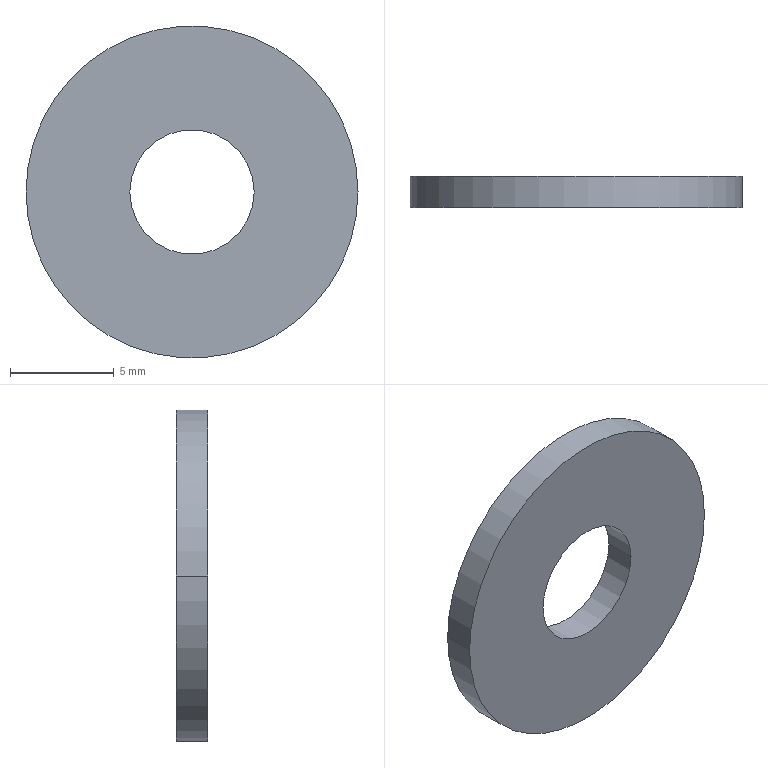Part | STEP file | WSSS16-6-1.5-3 | 1 solid | 6 faces | box 16 x 1.5 x 16 mm | volume 259.181 mm3 | cylinder 4 | plane 2 | commonest cylinder face diameters 6 x2 16 x2
STEP:
#1=CARTESIAN_POINT('',(0.,0.,0.));
#2=DIRECTION('',(0.,0.,1.));
#3=DIRECTION('',(1.,0.,0.));
#4=AXIS2_PLACEMENT_3D('',#1,#2,#3);
#5=CARTESIAN_POINT('',(-3.,0.,0.));
#6=VERTEX_POINT('',#5);
#7=CARTESIAN_POINT('',(-3.,1.5,0.));
#8=VERTEX_POINT('',#7);
#9=CARTESIAN_POINT('',(-3.,0.,0.));
#10=DIRECTION('',(0.,1.,0.));
#11=VECTOR('',#10,1.);
#12=LINE('',#9,#11);
#13=CARTESIAN_POINT('',(0.,0.,0.));
#14=DIRECTION('',(0.,1.,0.));
#15=DIRECTION('',(-1.,0.,0.));
#16=AXIS2_PLACEMENT_3D('',#13,#14,#15);
#17=CYLINDRICAL_SURFACE('',#16,3.);
#18=CARTESIAN_POINT('',(6.283,0.));
#19=DIRECTION('',(0.,1.));
#20=VECTOR('',#19,1.);
#21=LINE('',#18,#20);
#22=(GEOMETRIC_REPRESENTATION_CONTEXT(2)PARAMETRIC_REPRESENTATION_CONTEXT()REPRESENTATION_CONTEXT('',''));
#23=DEFINITIONAL_REPRESENTATION('',(#21),#22);
#24=PCURVE('',#17,#23);
#25=CARTESIAN_POINT('',(0.,0.,0.));
#26=DIRECTION('',(0.,1.,0.));
#27=DIRECTION('',(-1.,0.,0.));
#28=AXIS2_PLACEMENT_3D('',#25,#26,#27);
#29=CYLINDRICAL_SURFACE('',#28,3.);
#30=CARTESIAN_POINT('',(0.,0.));
#31=DIRECTION('',(0.,1.));
#32=VECTOR('',#31,1.);
#33=LINE('',#30,#32);
#34=(GEOMETRIC_REPRESENTATION_CONTEXT(2)PARAMETRIC_REPRESENTATION_CONTEXT()REPRESENTATION_CONTEXT('',''));
#35=DEFINITIONAL_REPRESENTATION('',(#33),#34);
#36=PCURVE('',#29,#35);
#37=SURFACE_CURVE('',#12,(#24,#36),.PCURVE_S1.);
#38=EDGE_CURVE('',#6,#8,#37,.T.);
#39=ORIENTED_EDGE('',*,*,#38,.T.);
#40=CARTESIAN_POINT('',(3.,1.5,0.));
#41=VERTEX_POINT('',#40);
#42=CARTESIAN_POINT('',(0.,1.5,0.));
#43=DIRECTION('',(0.,-1.,0.));
#44=DIRECTION('',(1.,0.,0.));
#45=AXIS2_PLACEMENT_3D('',#42,#43,#44);
#46=CIRCLE('',#45,3.);
#47=CARTESIAN_POINT('',(9.425,1.5));
#48=DIRECTION('',(-1.,0.));
#49=VECTOR('',#48,1.);
#50=LINE('',#47,#49);
#51=(GEOMETRIC_REPRESENTATION_CONTEXT(2)PARAMETRIC_REPRESENTATION_CONTEXT()REPRESENTATION_CONTEXT('',''));
#52=DEFINITIONAL_REPRESENTATION('',(#50),#51);
#53=PCURVE('',#17,#52);
#54=CARTESIAN_POINT('',(0.,1.5,0.));
#55=DIRECTION('',(0.,1.,0.));
#56=DIRECTION('',(-1.,0.,0.));
#57=AXIS2_PLACEMENT_3D('',#54,#55,#56);
#58=PLANE('',#57);
#59=CARTESIAN_POINT('',(-3.,0.));
#60=CARTESIAN_POINT('',(-3.,5.196));
#61=CARTESIAN_POINT('',(1.5,2.598));
#62=CARTESIAN_POINT('',(6.,0.));
#63=CARTESIAN_POINT('',(1.5,-2.598));
#64=CARTESIAN_POINT('',(-3.,-5.196));
#65=CARTESIAN_POINT('',(-3.,0.));
#66=(BOUNDED_CURVE()B_SPLINE_CURVE(2,(#59,#60,#61,#62,#63,#64,#65),.UNSPECIFIED.,.T.,.F.)B_SPLINE_CURVE_WITH_KNOTS((1,2,2,2,2,1),(-2.094,0.,2.094,4.189,6.283,8.378),.UNSPECIFIED.)CURVE()GEOMETRIC_REPRESENTATION_ITEM()RATIONAL_B_SPLINE_CURVE((1.,0.5,1.,0.5,1.,0.5,1.))REPRESENTATION_ITEM(''));
#67=(GEOMETRIC_REPRESENTATION_CONTEXT(2)PARAMETRIC_REPRESENTATION_CONTEXT()REPRESENTATION_CONTEXT('',''));
#68=DEFINITIONAL_REPRESENTATION('',(#66),#67);
#69=PCURVE('',#58,#68);
#70=SURFACE_CURVE('',#46,(#53,#69),.PCURVE_S1.);
#71=EDGE_CURVE('',#8,#41,#70,.T.);
#72=ORIENTED_EDGE('',*,*,#71,.T.);
#73=CARTESIAN_POINT('',(3.,0.,0.));
#74=VERTEX_POINT('',#73);
#75=CARTESIAN_POINT('',(3.,0.,0.));
#76=DIRECTION('',(0.,1.,0.));
#77=VECTOR('',#76,1.);
#78=LINE('',#75,#77);
#79=CARTESIAN_POINT('',(3.142,0.));
#80=DIRECTION('',(0.,1.));
#81=VECTOR('',#80,1.);
#82=LINE('',#79,#81);
#83=(GEOMETRIC_REPRESENTATION_CONTEXT(2)PARAMETRIC_REPRESENTATION_CONTEXT()REPRESENTATION_CONTEXT('',''));
#84=DEFINITIONAL_REPRESENTATION('',(#82),#83);
#85=PCURVE('',#17,#84);
#86=CARTESIAN_POINT('',(3.142,0.));
#87=DIRECTION('',(0.,1.));
#88=VECTOR('',#87,1.);
#89=LINE('',#86,#88);
#90=(GEOMETRIC_REPRESENTATION_CONTEXT(2)PARAMETRIC_REPRESENTATION_CONTEXT()REPRESENTATION_CONTEXT('',''));
#91=DEFINITIONAL_REPRESENTATION('',(#89),#90);
#92=PCURVE('',#29,#91);
#93=SURFACE_CURVE('',#78,(#85,#92),.PCURVE_S1.);
#94=EDGE_CURVE('',#74,#41,#93,.T.);
#95=ORIENTED_EDGE('',*,*,#94,.F.);
#96=CARTESIAN_POINT('',(0.,0.,0.));
#97=DIRECTION('',(0.,1.,0.));
#98=DIRECTION('',(-1.,0.,0.));
#99=AXIS2_PLACEMENT_3D('',#96,#97,#98);
#100=CIRCLE('',#99,3.);
#101=CARTESIAN_POINT('',(0.,0.));
#102=DIRECTION('',(1.,0.));
#103=VECTOR('',#102,1.);
#104=LINE('',#101,#103);
#105=(GEOMETRIC_REPRESENTATION_CONTEXT(2)PARAMETRIC_REPRESENTATION_CONTEXT()REPRESENTATION_CONTEXT('',''));
#106=DEFINITIONAL_REPRESENTATION('',(#104),#105);
#107=PCURVE('',#17,#106);
#108=CARTESIAN_POINT('',(0.,0.,0.));
#109=DIRECTION('',(0.,-1.,0.));
#110=DIRECTION('',(1.,0.,0.));
#111=AXIS2_PLACEMENT_3D('',#108,#109,#110);
#112=PLANE('',#111);
#113=CARTESIAN_POINT('',(-3.,0.));
#114=CARTESIAN_POINT('',(-3.,5.196));
#115=CARTESIAN_POINT('',(1.5,2.598));
#116=CARTESIAN_POINT('',(6.,0.));
#117=CARTESIAN_POINT('',(1.5,-2.598));
#118=CARTESIAN_POINT('',(-3.,-5.196));
#119=CARTESIAN_POINT('',(-3.,0.));
#120=(BOUNDED_CURVE()B_SPLINE_CURVE(2,(#113,#114,#115,#116,#117,#118,#119),.UNSPECIFIED.,.T.,.F.)B_SPLINE_CURVE_WITH_KNOTS((1,2,2,2,2,1),(-2.094,0.,2.094,4.189,6.283,8.378),.UNSPECIFIED.)CURVE()GEOMETRIC_REPRESENTATION_ITEM()RATIONAL_B_SPLINE_CURVE((1.,0.5,1.,0.5,1.,0.5,1.))REPRESENTATION_ITEM(''));
#121=(GEOMETRIC_REPRESENTATION_CONTEXT(2)PARAMETRIC_REPRESENTATION_CONTEXT()REPRESENTATION_CONTEXT('',''));
#122=DEFINITIONAL_REPRESENTATION('',(#120),#121);
#123=PCURVE('',#112,#122);
#124=SURFACE_CURVE('',#100,(#107,#123),.PCURVE_S1.);
#125=EDGE_CURVE('',#74,#6,#124,.T.);
#126=ORIENTED_EDGE('',*,*,#125,.T.);
#127=EDGE_LOOP('',(#39,#72,#95,#126));
#128=FACE_BOUND('',#127,.F.);
#129=ADVANCED_FACE('',(#128),#17,.F.);
#130=CARTESIAN_POINT('',(-8.,0.,0.));
#131=VERTEX_POINT('',#130);
#132=CARTESIAN_POINT('',(8.,0.,0.));
#133=VERTEX_POINT('',#132);
#134=CARTESIAN_POINT('',(0.,0.,0.));
#135=DIRECTION('',(0.,1.,0.));
#136=DIRECTION('',(-1.,0.,0.));
#137=AXIS2_PLACEMENT_3D('',#134,#135,#136);
#138=CIRCLE('',#137,8.);
#139=CARTESIAN_POINT('',(0.,0.,0.));
#140=DIRECTION('',(0.,1.,0.));
#141=DIRECTION('',(-1.,0.,0.));
#142=AXIS2_PLACEMENT_3D('',#139,#140,#141);
#143=CYLINDRICAL_SURFACE('',#142,8.);
#144=CARTESIAN_POINT('',(0.,0.));
#145=DIRECTION('',(1.,0.));
#146=VECTOR('',#145,1.);
#147=LINE('',#144,#146);
#148=(GEOMETRIC_REPRESENTATION_CONTEXT(2)PARAMETRIC_REPRESENTATION_CONTEXT()REPRESENTATION_CONTEXT('',''));
#149=DEFINITIONAL_REPRESENTATION('',(#147),#148);
#150=PCURVE('',#143,#149);
#151=CARTESIAN_POINT('',(-8.,0.));
#152=CARTESIAN_POINT('',(-8.,13.856));
#153=CARTESIAN_POINT('',(4.,6.928));
#154=CARTESIAN_POINT('',(16.,0.));
#155=CARTESIAN_POINT('',(4.,-6.928));
#156=CARTESIAN_POINT('',(-8.,-13.856));
#157=CARTESIAN_POINT('',(-8.,0.));
#158=(BOUNDED_CURVE()B_SPLINE_CURVE(2,(#151,#152,#153,#154,#155,#156,#157),.UNSPECIFIED.,.T.,.F.)B_SPLINE_CURVE_WITH_KNOTS((1,2,2,2,2,1),(-2.094,0.,2.094,4.189,6.283,8.378),.UNSPECIFIED.)CURVE()GEOMETRIC_REPRESENTATION_ITEM()RATIONAL_B_SPLINE_CURVE((1.,0.5,1.,0.5,1.,0.5,1.))REPRESENTATION_ITEM(''));
#159=(GEOMETRIC_REPRESENTATION_CONTEXT(2)PARAMETRIC_REPRESENTATION_CONTEXT()REPRESENTATION_CONTEXT('',''));
#160=DEFINITIONAL_REPRESENTATION('',(#158),#159);
#161=PCURVE('',#112,#160);
#162=SURFACE_CURVE('',#138,(#150,#161),.PCURVE_S1.);
#163=EDGE_CURVE('',#131,#133,#162,.T.);
#164=ORIENTED_EDGE('',*,*,#163,.T.);
#165=CARTESIAN_POINT('',(8.,1.5,0.));
#166=VERTEX_POINT('',#165);
#167=CARTESIAN_POINT('',(8.,0.,0.));
#168=DIRECTION('',(0.,1.,0.));
#169=VECTOR('',#168,1.);
#170=LINE('',#167,#169);
#171=CARTESIAN_POINT('',(3.142,0.));
#172=DIRECTION('',(0.,1.));
#173=VECTOR('',#172,1.);
#174=LINE('',#171,#173);
#175=(GEOMETRIC_REPRESENTATION_CONTEXT(2)PARAMETRIC_REPRESENTATION_CONTEXT()REPRESENTATION_CONTEXT('',''));
#176=DEFINITIONAL_REPRESENTATION('',(#174),#175);
#177=PCURVE('',#143,#176);
#178=CARTESIAN_POINT('',(0.,0.,0.));
#179=DIRECTION('',(0.,1.,0.));
#180=DIRECTION('',(-1.,0.,0.));
#181=AXIS2_PLACEMENT_3D('',#178,#179,#180);
#182=CYLINDRICAL_SURFACE('',#181,8.);
#183=CARTESIAN_POINT('',(3.142,0.));
#184=DIRECTION('',(0.,1.));
#185=VECTOR('',#184,1.);
#186=LINE('',#183,#185);
#187=(GEOMETRIC_REPRESENTATION_CONTEXT(2)PARAMETRIC_REPRESENTATION_CONTEXT()REPRESENTATION_CONTEXT('',''));
#188=DEFINITIONAL_REPRESENTATION('',(#186),#187);
#189=PCURVE('',#182,#188);
#190=SURFACE_CURVE('',#170,(#177,#189),.PCURVE_S1.);
#191=EDGE_CURVE('',#133,#166,#190,.T.);
#192=ORIENTED_EDGE('',*,*,#191,.T.);
#193=CARTESIAN_POINT('',(-8.,1.5,0.));
#194=VERTEX_POINT('',#193);
#195=CARTESIAN_POINT('',(0.,1.5,0.));
#196=DIRECTION('',(0.,-1.,0.));
#197=DIRECTION('',(1.,0.,0.));
#198=AXIS2_PLACEMENT_3D('',#195,#196,#197);
#199=CIRCLE('',#198,8.);
#200=CARTESIAN_POINT('',(3.142,1.5));
#201=DIRECTION('',(-1.,0.));
#202=VECTOR('',#201,1.);
#203=LINE('',#200,#202);
#204=(GEOMETRIC_REPRESENTATION_CONTEXT(2)PARAMETRIC_REPRESENTATION_CONTEXT()REPRESENTATION_CONTEXT('',''));
#205=DEFINITIONAL_REPRESENTATION('',(#203),#204);
#206=PCURVE('',#143,#205);
#207=CARTESIAN_POINT('',(-8.,0.));
#208=CARTESIAN_POINT('',(-8.,13.856));
#209=CARTESIAN_POINT('',(4.,6.928));
#210=CARTESIAN_POINT('',(16.,0.));
#211=CARTESIAN_POINT('',(4.,-6.928));
#212=CARTESIAN_POINT('',(-8.,-13.856));
#213=CARTESIAN_POINT('',(-8.,0.));
#214=(BOUNDED_CURVE()B_SPLINE_CURVE(2,(#207,#208,#209,#210,#211,#212,#213),.UNSPECIFIED.,.T.,.F.)B_SPLINE_CURVE_WITH_KNOTS((1,2,2,2,2,1),(-2.094,0.,2.094,4.189,6.283,8.378),.UNSPECIFIED.)CURVE()GEOMETRIC_REPRESENTATION_ITEM()RATIONAL_B_SPLINE_CURVE((1.,0.5,1.,0.5,1.,0.5,1.))REPRESENTATION_ITEM(''));
#215=(GEOMETRIC_REPRESENTATION_CONTEXT(2)PARAMETRIC_REPRESENTATION_CONTEXT()REPRESENTATION_CONTEXT('',''));
#216=DEFINITIONAL_REPRESENTATION('',(#214),#215);
#217=PCURVE('',#58,#216);
#218=SURFACE_CURVE('',#199,(#206,#217),.PCURVE_S1.);
#219=EDGE_CURVE('',#166,#194,#218,.T.);
#220=ORIENTED_EDGE('',*,*,#219,.T.);
#221=CARTESIAN_POINT('',(-8.,0.,0.));
#222=DIRECTION('',(0.,1.,0.));
#223=VECTOR('',#222,1.);
#224=LINE('',#221,#223);
#225=CARTESIAN_POINT('',(0.,0.));
#226=DIRECTION('',(0.,1.));
#227=VECTOR('',#226,1.);
#228=LINE('',#225,#227);
#229=(GEOMETRIC_REPRESENTATION_CONTEXT(2)PARAMETRIC_REPRESENTATION_CONTEXT()REPRESENTATION_CONTEXT('',''));
#230=DEFINITIONAL_REPRESENTATION('',(#228),#229);
#231=PCURVE('',#143,#230);
#232=CARTESIAN_POINT('',(6.283,0.));
#233=DIRECTION('',(0.,1.));
#234=VECTOR('',#233,1.);
#235=LINE('',#232,#234);
#236=(GEOMETRIC_REPRESENTATION_CONTEXT(2)PARAMETRIC_REPRESENTATION_CONTEXT()REPRESENTATION_CONTEXT('',''));
#237=DEFINITIONAL_REPRESENTATION('',(#235),#236);
#238=PCURVE('',#182,#237);
#239=SURFACE_CURVE('',#224,(#231,#238),.PCURVE_S1.);
#240=EDGE_CURVE('',#131,#194,#239,.T.);
#241=ORIENTED_EDGE('',*,*,#240,.F.);
#242=EDGE_LOOP('',(#164,#192,#220,#241));
#243=FACE_BOUND('',#242,.T.);
#244=ADVANCED_FACE('',(#243),#143,.T.);
#245=ORIENTED_EDGE('',*,*,#71,.T.);
#246=CARTESIAN_POINT('',(0.,1.5,0.));
#247=DIRECTION('',(0.,-1.,0.));
#248=DIRECTION('',(1.,0.,0.));
#249=AXIS2_PLACEMENT_3D('',#246,#247,#248);
#250=CIRCLE('',#249,3.);
#251=CARTESIAN_POINT('',(-3.,0.));
#252=CARTESIAN_POINT('',(-3.,5.196));
#253=CARTESIAN_POINT('',(1.5,2.598));
#254=CARTESIAN_POINT('',(6.,0.));
#255=CARTESIAN_POINT('',(1.5,-2.598));
#256=CARTESIAN_POINT('',(-3.,-5.196));
#257=CARTESIAN_POINT('',(-3.,0.));
#258=(BOUNDED_CURVE()B_SPLINE_CURVE(2,(#251,#252,#253,#254,#255,#256,#257),.UNSPECIFIED.,.T.,.F.)B_SPLINE_CURVE_WITH_KNOTS((1,2,2,2,2,1),(-2.094,0.,2.094,4.189,6.283,8.378),.UNSPECIFIED.)CURVE()GEOMETRIC_REPRESENTATION_ITEM()RATIONAL_B_SPLINE_CURVE((1.,0.5,1.,0.5,1.,0.5,1.))REPRESENTATION_ITEM(''));
#259=(GEOMETRIC_REPRESENTATION_CONTEXT(2)PARAMETRIC_REPRESENTATION_CONTEXT()REPRESENTATION_CONTEXT('',''));
#260=DEFINITIONAL_REPRESENTATION('',(#258),#259);
#261=PCURVE('',#58,#260);
#262=CARTESIAN_POINT('',(3.142,1.5));
#263=DIRECTION('',(-1.,0.));
#264=VECTOR('',#263,1.);
#265=LINE('',#262,#264);
#266=(GEOMETRIC_REPRESENTATION_CONTEXT(2)PARAMETRIC_REPRESENTATION_CONTEXT()REPRESENTATION_CONTEXT('',''));
#267=DEFINITIONAL_REPRESENTATION('',(#265),#266);
#268=PCURVE('',#29,#267);
#269=SURFACE_CURVE('',#250,(#261,#268),.PCURVE_S1.);
#270=EDGE_CURVE('',#41,#8,#269,.T.);
#271=ORIENTED_EDGE('',*,*,#270,.T.);
#272=EDGE_LOOP('',(#245,#271));
#273=FACE_BOUND('',#272,.T.);
#274=CARTESIAN_POINT('',(0.,1.5,0.));
#275=DIRECTION('',(0.,-1.,0.));
#276=DIRECTION('',(1.,0.,0.));
#277=AXIS2_PLACEMENT_3D('',#274,#275,#276);
#278=CIRCLE('',#277,8.);
#279=CARTESIAN_POINT('',(-8.,0.));
#280=CARTESIAN_POINT('',(-8.,13.856));
#281=CARTESIAN_POINT('',(4.,6.928));
#282=CARTESIAN_POINT('',(16.,0.));
#283=CARTESIAN_POINT('',(4.,-6.928));
#284=CARTESIAN_POINT('',(-8.,-13.856));
#285=CARTESIAN_POINT('',(-8.,0.));
#286=(BOUNDED_CURVE()B_SPLINE_CURVE(2,(#279,#280,#281,#282,#283,#284,#285),.UNSPECIFIED.,.T.,.F.)B_SPLINE_CURVE_WITH_KNOTS((1,2,2,2,2,1),(-2.094,0.,2.094,4.189,6.283,8.378),.UNSPECIFIED.)CURVE()GEOMETRIC_REPRESENTATION_ITEM()RATIONAL_B_SPLINE_CURVE((1.,0.5,1.,0.5,1.,0.5,1.))REPRESENTATION_ITEM(''));
#287=(GEOMETRIC_REPRESENTATION_CONTEXT(2)PARAMETRIC_REPRESENTATION_CONTEXT()REPRESENTATION_CONTEXT('',''));
#288=DEFINITIONAL_REPRESENTATION('',(#286),#287);
#289=PCURVE('',#58,#288);
#290=CARTESIAN_POINT('',(9.425,1.5));
#291=DIRECTION('',(-1.,0.));
#292=VECTOR('',#291,1.);
#293=LINE('',#290,#292);
#294=(GEOMETRIC_REPRESENTATION_CONTEXT(2)PARAMETRIC_REPRESENTATION_CONTEXT()REPRESENTATION_CONTEXT('',''));
#295=DEFINITIONAL_REPRESENTATION('',(#293),#294);
#296=PCURVE('',#182,#295);
#297=SURFACE_CURVE('',#278,(#289,#296),.PCURVE_S1.);
#298=EDGE_CURVE('',#194,#166,#297,.T.);
#299=ORIENTED_EDGE('',*,*,#298,.F.);
#300=ORIENTED_EDGE('',*,*,#219,.F.);
#301=EDGE_LOOP('',(#299,#300));
#302=FACE_BOUND('',#301,.T.);
#303=ADVANCED_FACE('',(#273,#302),#58,.T.);
#304=CARTESIAN_POINT('',(0.,0.,0.));
#305=DIRECTION('',(0.,1.,0.));
#306=DIRECTION('',(-1.,0.,0.));
#307=AXIS2_PLACEMENT_3D('',#304,#305,#306);
#308=CIRCLE('',#307,3.);
#309=CARTESIAN_POINT('',(-3.,0.));
#310=CARTESIAN_POINT('',(-3.,5.196));
#311=CARTESIAN_POINT('',(1.5,2.598));
#312=CARTESIAN_POINT('',(6.,0.));
#313=CARTESIAN_POINT('',(1.5,-2.598));
#314=CARTESIAN_POINT('',(-3.,-5.196));
#315=CARTESIAN_POINT('',(-3.,0.));
#316=(BOUNDED_CURVE()B_SPLINE_CURVE(2,(#309,#310,#311,#312,#313,#314,#315),.UNSPECIFIED.,.T.,.F.)B_SPLINE_CURVE_WITH_KNOTS((1,2,2,2,2,1),(-2.094,0.,2.094,4.189,6.283,8.378),.UNSPECIFIED.)CURVE()GEOMETRIC_REPRESENTATION_ITEM()RATIONAL_B_SPLINE_CURVE((1.,0.5,1.,0.5,1.,0.5,1.))REPRESENTATION_ITEM(''));
#317=(GEOMETRIC_REPRESENTATION_CONTEXT(2)PARAMETRIC_REPRESENTATION_CONTEXT()REPRESENTATION_CONTEXT('',''));
#318=DEFINITIONAL_REPRESENTATION('',(#316),#317);
#319=PCURVE('',#112,#318);
#320=CARTESIAN_POINT('',(0.,0.));
#321=DIRECTION('',(1.,0.));
#322=VECTOR('',#321,1.);
#323=LINE('',#320,#322);
#324=(GEOMETRIC_REPRESENTATION_CONTEXT(2)PARAMETRIC_REPRESENTATION_CONTEXT()REPRESENTATION_CONTEXT('',''));
#325=DEFINITIONAL_REPRESENTATION('',(#323),#324);
#326=PCURVE('',#29,#325);
#327=SURFACE_CURVE('',#308,(#319,#326),.PCURVE_S1.);
#328=EDGE_CURVE('',#6,#74,#327,.T.);
#329=ORIENTED_EDGE('',*,*,#328,.T.);
#330=ORIENTED_EDGE('',*,*,#125,.T.);
#331=EDGE_LOOP('',(#329,#330));
#332=FACE_BOUND('',#331,.T.);
#333=ORIENTED_EDGE('',*,*,#163,.F.);
#334=CARTESIAN_POINT('',(0.,0.,0.));
#335=DIRECTION('',(0.,1.,0.));
#336=DIRECTION('',(-1.,0.,0.));
#337=AXIS2_PLACEMENT_3D('',#334,#335,#336);
#338=CIRCLE('',#337,8.);
#339=CARTESIAN_POINT('',(-8.,0.));
#340=CARTESIAN_POINT('',(-8.,13.856));
#341=CARTESIAN_POINT('',(4.,6.928));
#342=CARTESIAN_POINT('',(16.,0.));
#343=CARTESIAN_POINT('',(4.,-6.928));
#344=CARTESIAN_POINT('',(-8.,-13.856));
#345=CARTESIAN_POINT('',(-8.,0.));
#346=(BOUNDED_CURVE()B_SPLINE_CURVE(2,(#339,#340,#341,#342,#343,#344,#345),.UNSPECIFIED.,.T.,.F.)B_SPLINE_CURVE_WITH_KNOTS((1,2,2,2,2,1),(-2.094,0.,2.094,4.189,6.283,8.378),.UNSPECIFIED.)CURVE()GEOMETRIC_REPRESENTATION_ITEM()RATIONAL_B_SPLINE_CURVE((1.,0.5,1.,0.5,1.,0.5,1.))REPRESENTATION_ITEM(''));
#347=(GEOMETRIC_REPRESENTATION_CONTEXT(2)PARAMETRIC_REPRESENTATION_CONTEXT()REPRESENTATION_CONTEXT('',''));
#348=DEFINITIONAL_REPRESENTATION('',(#346),#347);
#349=PCURVE('',#112,#348);
#350=CARTESIAN_POINT('',(0.,0.));
#351=DIRECTION('',(1.,0.));
#352=VECTOR('',#351,1.);
#353=LINE('',#350,#352);
#354=(GEOMETRIC_REPRESENTATION_CONTEXT(2)PARAMETRIC_REPRESENTATION_CONTEXT()REPRESENTATION_CONTEXT('',''));
#355=DEFINITIONAL_REPRESENTATION('',(#353),#354);
#356=PCURVE('',#182,#355);
#357=SURFACE_CURVE('',#338,(#349,#356),.PCURVE_S1.);
#358=EDGE_CURVE('',#133,#131,#357,.T.);
#359=ORIENTED_EDGE('',*,*,#358,.F.);
#360=EDGE_LOOP('',(#333,#359));
#361=FACE_BOUND('',#360,.T.);
#362=ADVANCED_FACE('',(#332,#361),#112,.T.);
#363=ORIENTED_EDGE('',*,*,#191,.F.);
#364=ORIENTED_EDGE('',*,*,#358,.T.);
#365=ORIENTED_EDGE('',*,*,#240,.T.);
#366=ORIENTED_EDGE('',*,*,#298,.T.);
#367=EDGE_LOOP('',(#363,#364,#365,#366));
#368=FACE_BOUND('',#367,.T.);
#369=ADVANCED_FACE('',(#368),#182,.T.);
#370=ORIENTED_EDGE('',*,*,#270,.T.);
#371=ORIENTED_EDGE('',*,*,#38,.F.);
#372=ORIENTED_EDGE('',*,*,#328,.T.);
#373=ORIENTED_EDGE('',*,*,#94,.T.);
#374=EDGE_LOOP('',(#370,#371,#372,#373));
#375=FACE_BOUND('',#374,.F.);
#376=ADVANCED_FACE('',(#375),#29,.F.);
#377=CLOSED_SHELL('',(#129,#244,#303,#362,#369,#376));
#378=MANIFOLD_SOLID_BREP('',#377);
#379=(LENGTH_UNIT()NAMED_UNIT(*)SI_UNIT(.MILLI.,.METRE.));
#380=UNCERTAINTY_MEASURE_WITH_UNIT(LENGTH_MEASURE(0.0000001),#379,'','');
#381=(NAMED_UNIT(*)PLANE_ANGLE_UNIT()SI_UNIT($,.RADIAN.));
#382=(NAMED_UNIT(*)SI_UNIT($,.STERADIAN.)SOLID_ANGLE_UNIT());
#383=(GEOMETRIC_REPRESENTATION_CONTEXT(3)GLOBAL_UNCERTAINTY_ASSIGNED_CONTEXT((#380))GLOBAL_UNIT_ASSIGNED_CONTEXT((#379,#381,#382))REPRESENTATION_CONTEXT('',''));
#384=ADVANCED_BREP_SHAPE_REPRESENTATION('',(#4,#378),#383);